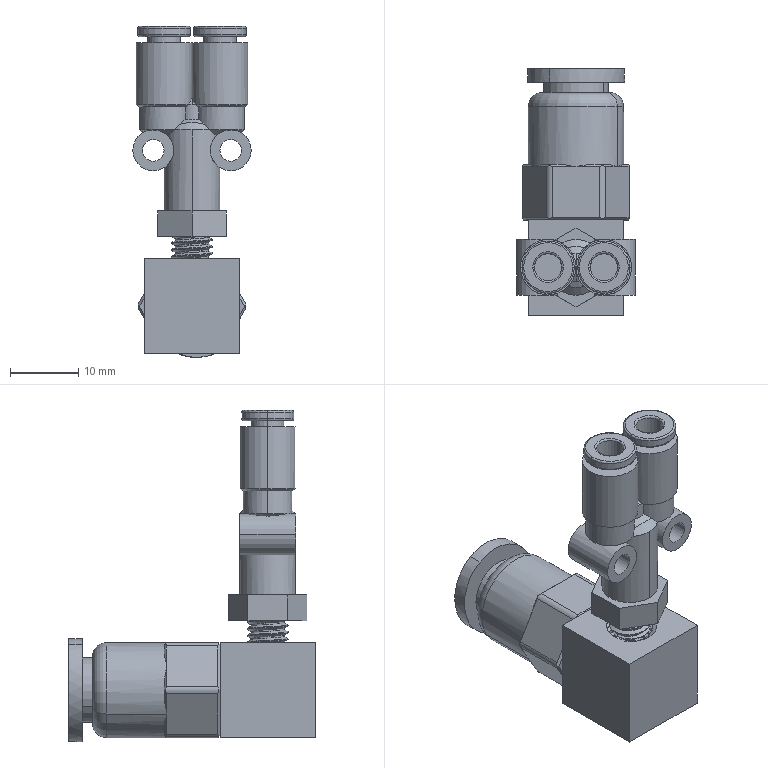Part | SolidWorks | 7 solids | 285 faces | box 17.4 x 36.23 x 48.652 mm | volume 7597 mm3 | cylinder 160 | plane 72 | torus 18 | cone 16 | spline 15 | sphere 4 | commonest cylinder face diameters 7.866 x19 6.446 x18 8.17 x14 6 x12 7.779 x12 9.17 x12